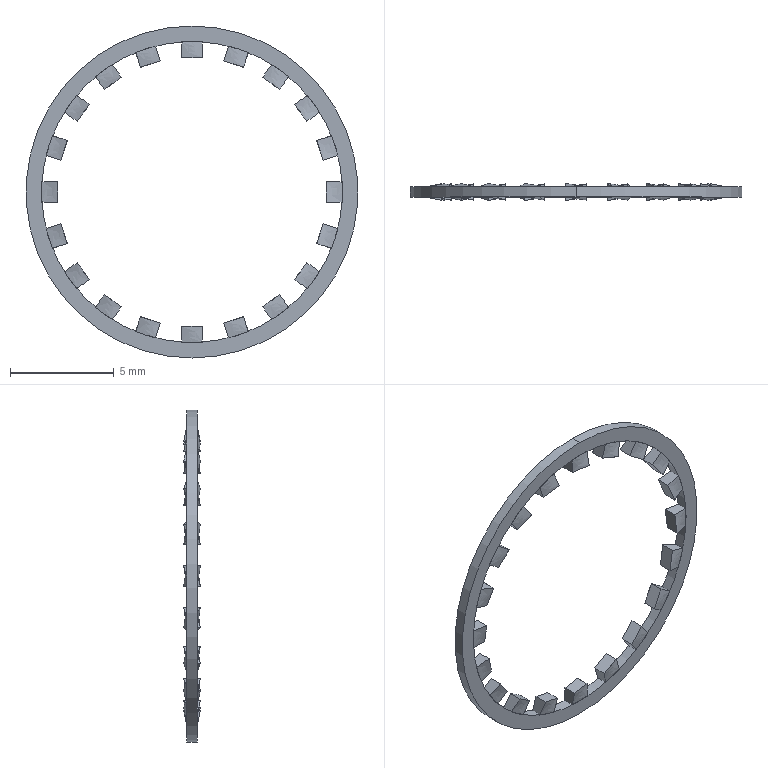Part | SolidWorks | features 3DProfileFeature 10, FillRefSurface 5, CirPattern 1, Extrusion 1, SewRefSurface 1, Thicken 1 | 21 solids | 286 faces | box 16 x 0.8028 x 16 mm | volume 17.966 mm3 | spline 180 | plane 102 | cylinder 4 | commonest cylinder face diameters 14.5 x2 16 x2